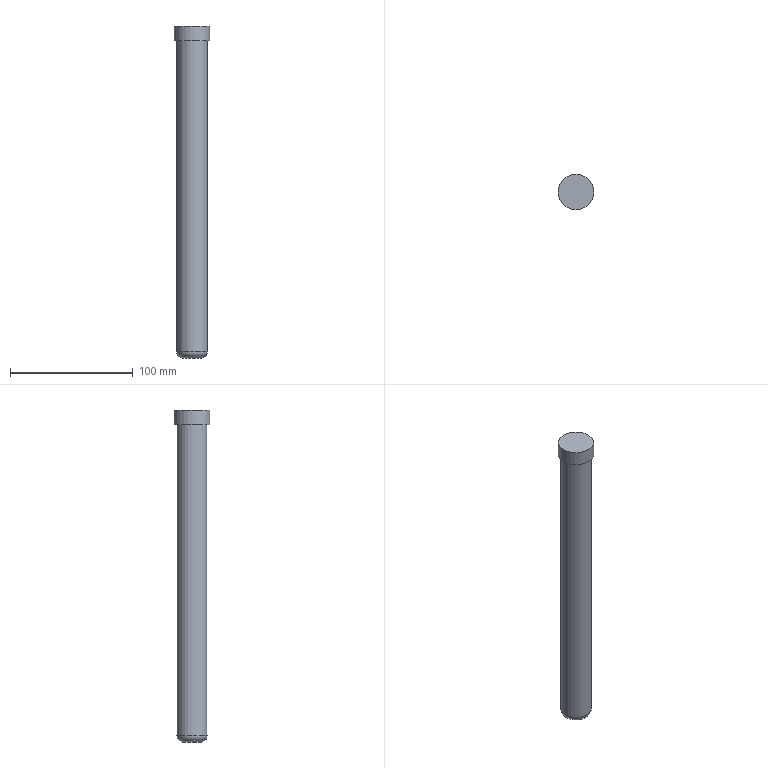Part | STEP file | lll_id522_x_t | 1 solid | 6 faces | box 29 x 29 x 271 mm | volume 134679 mm3 | plane 3 | cylinder 2 | torus 1 | commonest cylinder face diameters 25 x1 29 x1
STEP:
#1=CARTESIAN_POINT('',(-82.5,-117.,155.5));
#2=VERTEX_POINT('',#1);
#3=CARTESIAN_POINT('',(-97.,-117.,155.5));
#4=DIRECTION('',(0.,0.,-1.));
#5=DIRECTION('',(1.,0.,0.));
#6=AXIS2_PLACEMENT_3D('',#3,#4,#5);
#7=CIRCLE('',#6,14.5);
#8=EDGE_CURVE('',#2,#2,#7,.T.);
#9=ORIENTED_EDGE('',*,*,#8,.F.);
#10=EDGE_LOOP('',(#9));
#11=FACE_OUTER_BOUND('',#10,.T.);
#12=CARTESIAN_POINT('',(0.,0.,155.5));
#13=DIRECTION('',(0.,0.,1.));
#14=DIRECTION('',(1.,0.,0.));
#15=AXIS2_PLACEMENT_3D('',#12,#13,#14);
#16=PLANE('',#15);
#17=ADVANCED_FACE('',(#11),#16,.T.);
#18=CARTESIAN_POINT('',(-84.5,-117.,143.5));
#19=VERTEX_POINT('',#18);
#20=CARTESIAN_POINT('',(-97.,-117.,143.5));
#21=DIRECTION('',(0.,0.,1.));
#22=DIRECTION('',(1.,0.,0.));
#23=AXIS2_PLACEMENT_3D('',#20,#21,#22);
#24=CIRCLE('',#23,12.5);
#25=EDGE_CURVE('',#19,#19,#24,.T.);
#26=ORIENTED_EDGE('',*,*,#25,.T.);
#27=EDGE_LOOP('',(#26));
#28=FACE_BOUND('',#27,.T.);
#29=CARTESIAN_POINT('',(-111.5,-117.,143.5));
#30=VERTEX_POINT('',#29);
#31=CARTESIAN_POINT('',(-97.,-117.,143.5));
#32=DIRECTION('',(0.,0.,-1.));
#33=DIRECTION('',(-1.,0.,0.));
#34=AXIS2_PLACEMENT_3D('',#31,#32,#33);
#35=CIRCLE('',#34,14.5);
#36=EDGE_CURVE('',#30,#30,#35,.T.);
#37=ORIENTED_EDGE('',*,*,#36,.T.);
#38=EDGE_LOOP('',(#37));
#39=FACE_BOUND('',#38,.T.);
#40=CARTESIAN_POINT('',(-97.,-117.,143.5));
#41=DIRECTION('',(0.,0.,-1.));
#42=DIRECTION('',(-1.,0.,0.));
#43=AXIS2_PLACEMENT_3D('',#40,#41,#42);
#44=PLANE('',#43);
#45=ADVANCED_FACE('',(#28,#39),#44,.T.);
#46=ORIENTED_EDGE('',*,*,#36,.F.);
#47=EDGE_LOOP('',(#46));
#48=FACE_BOUND('',#47,.T.);
#49=ORIENTED_EDGE('',*,*,#8,.T.);
#50=EDGE_LOOP('',(#49));
#51=FACE_BOUND('',#50,.T.);
#52=CARTESIAN_POINT('',(-97.,-117.,262.3));
#53=DIRECTION('',(0.,0.,-1.));
#54=DIRECTION('',(-1.,0.,0.));
#55=AXIS2_PLACEMENT_3D('',#52,#53,#54);
#56=CYLINDRICAL_SURFACE('',#55,14.5);
#57=ADVANCED_FACE('',(#48,#51),#56,.T.);
#58=CARTESIAN_POINT('',(-89.5,-117.,-115.5));
#59=VERTEX_POINT('',#58);
#60=CARTESIAN_POINT('',(-97.,-117.,-115.5));
#61=DIRECTION('',(0.,0.,-1.));
#62=DIRECTION('',(1.,0.,0.));
#63=AXIS2_PLACEMENT_3D('',#60,#61,#62);
#64=CIRCLE('',#63,7.5);
#65=EDGE_CURVE('',#59,#59,#64,.T.);
#66=ORIENTED_EDGE('',*,*,#65,.T.);
#67=EDGE_LOOP('',(#66));
#68=FACE_OUTER_BOUND('',#67,.T.);
#69=CARTESIAN_POINT('',(0.,0.,-115.5));
#70=DIRECTION('',(0.,0.,1.));
#71=DIRECTION('',(1.,0.,0.));
#72=AXIS2_PLACEMENT_3D('',#69,#70,#71);
#73=PLANE('',#72);
#74=ADVANCED_FACE('',(#68),#73,.F.);
#75=CARTESIAN_POINT('',(-84.5,-117.,-110.5));
#76=VERTEX_POINT('',#75);
#77=CARTESIAN_POINT('',(-97.,-117.,-110.5));
#78=DIRECTION('',(0.,0.,1.));
#79=DIRECTION('',(1.,0.,0.));
#80=AXIS2_PLACEMENT_3D('',#77,#78,#79);
#81=CIRCLE('',#80,12.5);
#82=EDGE_CURVE('',#76,#76,#81,.T.);
#83=ORIENTED_EDGE('',*,*,#82,.T.);
#84=EDGE_LOOP('',(#83));
#85=FACE_BOUND('',#84,.T.);
#86=ORIENTED_EDGE('',*,*,#25,.F.);
#87=EDGE_LOOP('',(#86));
#88=FACE_BOUND('',#87,.T.);
#89=CARTESIAN_POINT('',(-97.,-117.,-2420.589));
#90=DIRECTION('',(0.,0.,1.));
#91=DIRECTION('',(1.,0.,0.));
#92=AXIS2_PLACEMENT_3D('',#89,#90,#91);
#93=CYLINDRICAL_SURFACE('',#92,12.5);
#94=ADVANCED_FACE('',(#85,#88),#93,.T.);
#95=ORIENTED_EDGE('',*,*,#82,.F.);
#96=EDGE_LOOP('',(#95));
#97=FACE_BOUND('',#96,.T.);
#98=ORIENTED_EDGE('',*,*,#65,.F.);
#99=EDGE_LOOP('',(#98));
#100=FACE_BOUND('',#99,.T.);
#101=CARTESIAN_POINT('',(-97.,-117.,-110.5));
#102=DIRECTION('',(0.,0.,1.));
#103=DIRECTION('',(1.,0.,0.));
#104=AXIS2_PLACEMENT_3D('',#101,#102,#103);
#105=TOROIDAL_SURFACE('',#104,7.5,5.);
#106=ADVANCED_FACE('',(#97,#100),#105,.T.);
#107=CLOSED_SHELL('',(#17,#45,#57,#74,#94,#106));
#108=MANIFOLD_SOLID_BREP('',#107);
#109=(LENGTH_UNIT()NAMED_UNIT(*)SI_UNIT(.MILLI.,.METRE.));
#110=UNCERTAINTY_MEASURE_WITH_UNIT(LENGTH_MEASURE(0.00002),#109,'','');
#111=(NAMED_UNIT(*)PLANE_ANGLE_UNIT()SI_UNIT($,.RADIAN.));
#112=PLANE_ANGLE_MEASURE_WITH_UNIT(PLANE_ANGLE_MEASURE(0.01745),#111);
#113=DIMENSIONAL_EXPONENTS(0.,0.,0.,0.,0.,0.,0.);
#114=(CONVERSION_BASED_UNIT('DEGREE',#112)NAMED_UNIT(#113)PLANE_ANGLE_UNIT());
#115=(NAMED_UNIT(*)SI_UNIT($,.STERADIAN.)SOLID_ANGLE_UNIT());
#116=(GEOMETRIC_REPRESENTATION_CONTEXT(3)GLOBAL_UNCERTAINTY_ASSIGNED_CONTEXT((#110))GLOBAL_UNIT_ASSIGNED_CONTEXT((#109,#114,#115))REPRESENTATION_CONTEXT('',''));
#117=ADVANCED_BREP_SHAPE_REPRESENTATION('',(#108),#116);